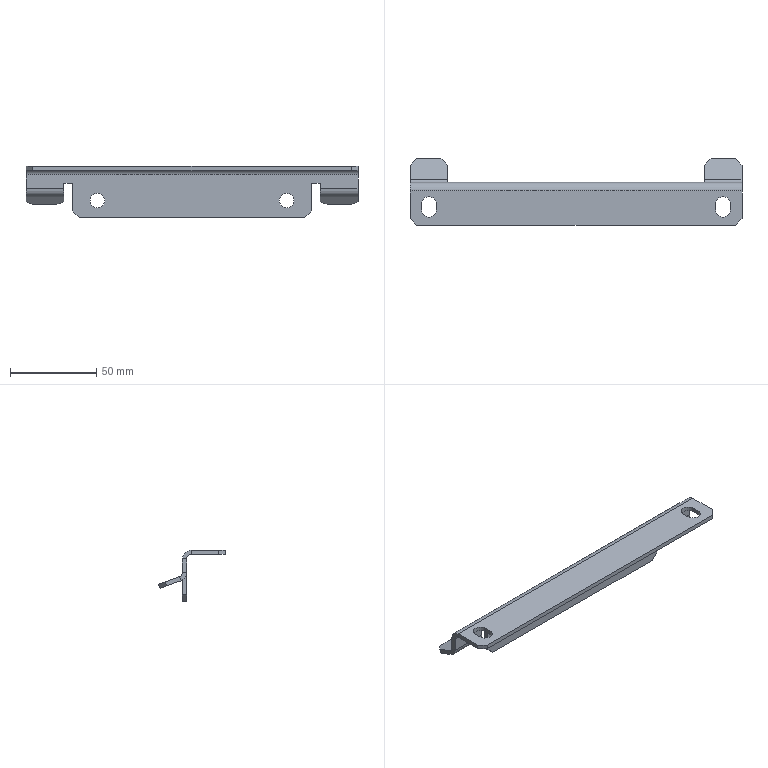Part | STEP file | 64668005 | 1 solid | 58 faces | box 193 x 38.839 x 30 mm | volume 23240 mm3 | plane 44 | cylinder 14 | commonest cylinder face diameters 8.5 x8 5 x3 10 x3